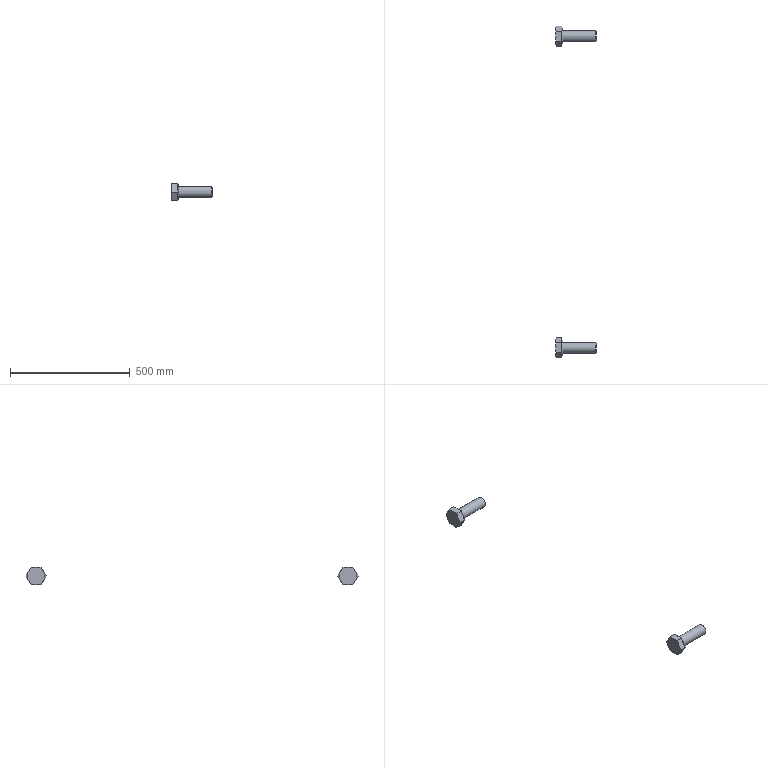Part | NX | features 10.SLDPRT 2, Delete Body 1, LINKED_BODY 1, SCALE 1 | 2 solids | 38 faces | box 170.438 x 1384 x 73.125 mm | volume 715384 mm3 | plane 20 | cone 16 | cylinder 2 | commonest cylinder face diameters 45 x2
STEP:
#1=CARTESIAN_POINT('',(351.807,1380.604,39.509));
#2=VERTEX_POINT('',#1);
#3=CARTESIAN_POINT('',(351.807,1380.604,7.25));
#4=DIRECTION('',(-1.,0.,0.));
#5=DIRECTION('',(0.,0.,1.));
#6=AXIS2_PLACEMENT_3D('',#3,#4,#5);
#7=CIRCLE('',#6,32.259);
#8=EDGE_CURVE('',#2,#2,#7,.T.);
#9=ORIENTED_EDGE('',*,*,#8,.F.);
#10=EDGE_LOOP('',(#9));
#11=FACE_BOUND('',#10,.T.);
#12=CARTESIAN_POINT('',(351.807,1380.604,29.75));
#13=VERTEX_POINT('',#12);
#14=CARTESIAN_POINT('',(351.807,1380.604,7.25));
#15=DIRECTION('',(-1.,0.,0.));
#16=DIRECTION('',(0.,0.,1.));
#17=AXIS2_PLACEMENT_3D('',#14,#15,#16);
#18=CIRCLE('',#17,22.5);
#19=EDGE_CURVE('',#13,#13,#18,.F.);
#20=ORIENTED_EDGE('',*,*,#19,.F.);
#21=EDGE_LOOP('',(#20));
#22=FACE_BOUND('',#21,.T.);
#23=CARTESIAN_POINT('',(351.807,1359.495,43.812));
#24=DIRECTION('',(-1.,0.,0.));
#25=DIRECTION('',(0.,0.,1.));
#26=AXIS2_PLACEMENT_3D('',#23,#24,#25);
#27=PLANE('',#26);
#28=ADVANCED_FACE('',(#11,#22),#27,.F.);
#29=CARTESIAN_POINT('',(324.054,1338.386,7.25));
#30=VERTEX_POINT('',#29);
#31=CARTESIAN_POINT('',(321.995,1348.94,25.531));
#32=VERTEX_POINT('',#31);
#33=CARTESIAN_POINT('',(324.054,1338.386,7.25));
#34=CARTESIAN_POINT('',(322.773,1341.904,13.344));
#35=CARTESIAN_POINT('',(321.995,1345.422,19.438));
#36=CARTESIAN_POINT('',(321.995,1348.94,25.531));
#37=B_SPLINE_CURVE_WITH_KNOTS('',3,(#33,#34,#35,#36),.UNSPECIFIED.,.F.,.F.,(4,4),(0.000001299,0.02111),.UNSPECIFIED.);
#38=EDGE_CURVE('',#30,#32,#37,.T.);
#39=ORIENTED_EDGE('',*,*,#38,.F.);
#40=CARTESIAN_POINT('',(348.432,1338.386,7.25));
#41=VERTEX_POINT('',#40);
#42=CARTESIAN_POINT('',(351.807,1338.386,7.25));
#43=DIRECTION('',(-1.,0.,0.));
#44=VECTOR('',#43,1000.);
#45=LINE('',#42,#44);
#46=EDGE_CURVE('',#41,#30,#45,.T.);
#47=ORIENTED_EDGE('',*,*,#46,.F.);
#48=CARTESIAN_POINT('',(348.432,1359.495,43.812));
#49=VERTEX_POINT('',#48);
#50=CARTESIAN_POINT('',(348.432,1359.495,43.812));
#51=DIRECTION('',(0.,-0.5,-0.866));
#52=VECTOR('',#51,1000.);
#53=LINE('',#50,#52);
#54=EDGE_CURVE('',#49,#41,#53,.T.);
#55=ORIENTED_EDGE('',*,*,#54,.F.);
#56=CARTESIAN_POINT('',(324.054,1359.495,43.812));
#57=VERTEX_POINT('',#56);
#58=CARTESIAN_POINT('',(351.807,1359.495,43.812));
#59=DIRECTION('',(-1.,0.,0.));
#60=VECTOR('',#59,1000.);
#61=LINE('',#58,#60);
#62=EDGE_CURVE('',#49,#57,#61,.T.);
#63=ORIENTED_EDGE('',*,*,#62,.T.);
#64=CARTESIAN_POINT('',(321.995,1348.94,25.531));
#65=CARTESIAN_POINT('',(321.995,1352.459,31.625));
#66=CARTESIAN_POINT('',(322.773,1355.977,37.719));
#67=CARTESIAN_POINT('',(324.054,1359.495,43.813));
#68=B_SPLINE_CURVE_WITH_KNOTS('',3,(#64,#65,#66,#67),.UNSPECIFIED.,.F.,.F.,(4,4),(0.02111,0.04222),.UNSPECIFIED.);
#69=EDGE_CURVE('',#32,#57,#68,.T.);
#70=ORIENTED_EDGE('',*,*,#69,.F.);
#71=EDGE_LOOP('',(#39,#47,#55,#63,#70));
#72=FACE_BOUND('',#71,.T.);
#73=CARTESIAN_POINT('',(351.807,1359.495,43.812));
#74=DIRECTION('',(0.,0.866,-0.5));
#75=DIRECTION('',(0.,0.5,0.866));
#76=AXIS2_PLACEMENT_3D('',#73,#74,#75);
#77=PLANE('',#76);
#78=ADVANCED_FACE('',(#72),#77,.F.);
#79=CARTESIAN_POINT('',(324.054,1359.495,-29.312));
#80=VERTEX_POINT('',#79);
#81=CARTESIAN_POINT('',(321.995,1348.94,-11.031));
#82=VERTEX_POINT('',#81);
#83=CARTESIAN_POINT('',(324.054,1359.495,-29.312));
#84=CARTESIAN_POINT('',(322.773,1355.977,-23.219));
#85=CARTESIAN_POINT('',(321.995,1352.459,-17.125));
#86=CARTESIAN_POINT('',(321.995,1348.94,-11.031));
#87=B_SPLINE_CURVE_WITH_KNOTS('',3,(#83,#84,#85,#86),.UNSPECIFIED.,.F.,.F.,(4,4),(0.000001299,0.02111),.UNSPECIFIED.);
#88=EDGE_CURVE('',#80,#82,#87,.T.);
#89=ORIENTED_EDGE('',*,*,#88,.F.);
#90=CARTESIAN_POINT('',(348.432,1359.495,-29.312));
#91=VERTEX_POINT('',#90);
#92=CARTESIAN_POINT('',(351.807,1359.495,-29.312));
#93=DIRECTION('',(-1.,0.,0.));
#94=VECTOR('',#93,1000.);
#95=LINE('',#92,#94);
#96=EDGE_CURVE('',#91,#80,#95,.T.);
#97=ORIENTED_EDGE('',*,*,#96,.F.);
#98=CARTESIAN_POINT('',(348.432,1338.386,7.25));
#99=DIRECTION('',(0.,0.5,-0.866));
#100=VECTOR('',#99,1000.);
#101=LINE('',#98,#100);
#102=EDGE_CURVE('',#41,#91,#101,.T.);
#103=ORIENTED_EDGE('',*,*,#102,.F.);
#104=ORIENTED_EDGE('',*,*,#46,.T.);
#105=CARTESIAN_POINT('',(321.995,1348.94,-11.031));
#106=CARTESIAN_POINT('',(321.995,1345.422,-4.937));
#107=CARTESIAN_POINT('',(322.773,1341.904,1.156));
#108=CARTESIAN_POINT('',(324.054,1338.386,7.25));
#109=B_SPLINE_CURVE_WITH_KNOTS('',3,(#105,#106,#107,#108),.UNSPECIFIED.,.F.,.F.,(4,4),(0.02111,0.04222),.UNSPECIFIED.);
#110=EDGE_CURVE('',#82,#30,#109,.T.);
#111=ORIENTED_EDGE('',*,*,#110,.F.);
#112=EDGE_LOOP('',(#89,#97,#103,#104,#111));
#113=FACE_BOUND('',#112,.T.);
#114=CARTESIAN_POINT('',(351.807,1338.386,7.25));
#115=DIRECTION('',(0.,0.866,0.5));
#116=DIRECTION('',(0.,-0.5,0.866));
#117=AXIS2_PLACEMENT_3D('',#114,#115,#116);
#118=PLANE('',#117);
#119=ADVANCED_FACE('',(#113),#118,.F.);
#120=CARTESIAN_POINT('',(324.054,1401.714,-29.312));
#121=VERTEX_POINT('',#120);
#122=CARTESIAN_POINT('',(321.995,1380.604,-29.312));
#123=VERTEX_POINT('',#122);
#124=CARTESIAN_POINT('',(321.995,1380.604,-29.312));
#125=CARTESIAN_POINT('',(321.995,1387.655,-29.312));
#126=CARTESIAN_POINT('',(322.777,1394.696,-29.312));
#127=CARTESIAN_POINT('',(324.054,1401.714,-29.312));
#128=B_SPLINE_CURVE_WITH_KNOTS('',3,(#124,#125,#126,#127),.UNSPECIFIED.,.F.,.F.,(4,4),(0.05719,0.07852),.UNSPECIFIED.);
#129=EDGE_CURVE('',#121,#123,#128,.F.);
#130=ORIENTED_EDGE('',*,*,#129,.F.);
#131=CARTESIAN_POINT('',(348.432,1401.714,-29.312));
#132=VERTEX_POINT('',#131);
#133=CARTESIAN_POINT('',(351.807,1401.714,-29.312));
#134=DIRECTION('',(-1.,0.,0.));
#135=VECTOR('',#134,1000.);
#136=LINE('',#133,#135);
#137=EDGE_CURVE('',#132,#121,#136,.T.);
#138=ORIENTED_EDGE('',*,*,#137,.F.);
#139=CARTESIAN_POINT('',(348.432,1359.495,-29.312));
#140=DIRECTION('',(0.,1.,0.));
#141=VECTOR('',#140,1000.);
#142=LINE('',#139,#141);
#143=EDGE_CURVE('',#91,#132,#142,.T.);
#144=ORIENTED_EDGE('',*,*,#143,.F.);
#145=ORIENTED_EDGE('',*,*,#96,.T.);
#146=CARTESIAN_POINT('',(324.054,1359.495,-29.312));
#147=CARTESIAN_POINT('',(322.782,1366.485,-29.312));
#148=CARTESIAN_POINT('',(321.995,1373.574,-29.312));
#149=CARTESIAN_POINT('',(321.995,1380.604,-29.312));
#150=B_SPLINE_CURVE_WITH_KNOTS('',3,(#146,#147,#148,#149),.UNSPECIFIED.,.F.,.F.,(4,4),(0.03591,0.05719),.UNSPECIFIED.);
#151=EDGE_CURVE('',#123,#80,#150,.F.);
#152=ORIENTED_EDGE('',*,*,#151,.F.);
#153=EDGE_LOOP('',(#130,#138,#144,#145,#152));
#154=FACE_BOUND('',#153,.T.);
#155=CARTESIAN_POINT('',(351.807,1359.495,-29.312));
#156=DIRECTION('',(0.,0.,1.));
#157=DIRECTION('',(0.,-1.,0.));
#158=AXIS2_PLACEMENT_3D('',#155,#156,#157);
#159=PLANE('',#158);
#160=ADVANCED_FACE('',(#154),#159,.F.);
#161=CARTESIAN_POINT('',(324.054,1422.823,7.25));
#162=VERTEX_POINT('',#161);
#163=CARTESIAN_POINT('',(321.995,1412.268,-11.031));
#164=VERTEX_POINT('',#163);
#165=CARTESIAN_POINT('',(324.054,1422.823,7.25));
#166=CARTESIAN_POINT('',(322.773,1419.305,1.156));
#167=CARTESIAN_POINT('',(321.995,1415.787,-4.938));
#168=CARTESIAN_POINT('',(321.995,1412.268,-11.031));
#169=B_SPLINE_CURVE_WITH_KNOTS('',3,(#165,#166,#167,#168),.UNSPECIFIED.,.F.,.F.,(4,4),(0.000001299,0.02111),.UNSPECIFIED.);
#170=EDGE_CURVE('',#162,#164,#169,.T.);
#171=ORIENTED_EDGE('',*,*,#170,.F.);
#172=CARTESIAN_POINT('',(348.432,1422.823,7.25));
#173=VERTEX_POINT('',#172);
#174=CARTESIAN_POINT('',(351.807,1422.823,7.25));
#175=DIRECTION('',(-1.,0.,0.));
#176=VECTOR('',#175,1000.);
#177=LINE('',#174,#176);
#178=EDGE_CURVE('',#173,#162,#177,.T.);
#179=ORIENTED_EDGE('',*,*,#178,.F.);
#180=CARTESIAN_POINT('',(348.432,1401.714,-29.312));
#181=DIRECTION('',(0.,0.5,0.866));
#182=VECTOR('',#181,1000.);
#183=LINE('',#180,#182);
#184=EDGE_CURVE('',#132,#173,#183,.T.);
#185=ORIENTED_EDGE('',*,*,#184,.F.);
#186=ORIENTED_EDGE('',*,*,#137,.T.);
#187=CARTESIAN_POINT('',(321.995,1412.268,-11.031));
#188=CARTESIAN_POINT('',(321.995,1408.75,-17.125));
#189=CARTESIAN_POINT('',(322.773,1405.232,-23.219));
#190=CARTESIAN_POINT('',(324.054,1401.714,-29.312));
#191=B_SPLINE_CURVE_WITH_KNOTS('',3,(#187,#188,#189,#190),.UNSPECIFIED.,.F.,.F.,(4,4),(0.02111,0.04222),.UNSPECIFIED.);
#192=EDGE_CURVE('',#164,#121,#191,.T.);
#193=ORIENTED_EDGE('',*,*,#192,.F.);
#194=EDGE_LOOP('',(#171,#179,#185,#186,#193));
#195=FACE_BOUND('',#194,.T.);
#196=CARTESIAN_POINT('',(351.807,1401.714,-29.312));
#197=DIRECTION('',(0.,-0.866,0.5));
#198=DIRECTION('',(0.,-0.5,-0.866));
#199=AXIS2_PLACEMENT_3D('',#196,#197,#198);
#200=PLANE('',#199);
#201=ADVANCED_FACE('',(#195),#200,.F.);
#202=CARTESIAN_POINT('',(324.054,1401.714,43.812));
#203=VERTEX_POINT('',#202);
#204=CARTESIAN_POINT('',(321.995,1412.268,25.531));
#205=VERTEX_POINT('',#204);
#206=CARTESIAN_POINT('',(324.054,1401.714,43.812));
#207=CARTESIAN_POINT('',(322.773,1405.232,37.719));
#208=CARTESIAN_POINT('',(321.995,1408.75,31.625));
#209=CARTESIAN_POINT('',(321.995,1412.268,25.531));
#210=B_SPLINE_CURVE_WITH_KNOTS('',3,(#206,#207,#208,#209),.UNSPECIFIED.,.F.,.F.,(4,4),(0.000001299,0.02111),.UNSPECIFIED.);
#211=EDGE_CURVE('',#203,#205,#210,.T.);
#212=ORIENTED_EDGE('',*,*,#211,.F.);
#213=CARTESIAN_POINT('',(348.432,1401.714,43.812));
#214=VERTEX_POINT('',#213);
#215=CARTESIAN_POINT('',(351.807,1401.714,43.812));
#216=DIRECTION('',(-1.,0.,0.));
#217=VECTOR('',#216,1000.);
#218=LINE('',#215,#217);
#219=EDGE_CURVE('',#214,#203,#218,.T.);
#220=ORIENTED_EDGE('',*,*,#219,.F.);
#221=CARTESIAN_POINT('',(348.432,1422.823,7.25));
#222=DIRECTION('',(0.,-0.5,0.866));
#223=VECTOR('',#222,1000.);
#224=LINE('',#221,#223);
#225=EDGE_CURVE('',#173,#214,#224,.T.);
#226=ORIENTED_EDGE('',*,*,#225,.F.);
#227=ORIENTED_EDGE('',*,*,#178,.T.);
#228=CARTESIAN_POINT('',(321.995,1412.268,25.531));
#229=CARTESIAN_POINT('',(321.995,1415.787,19.438));
#230=CARTESIAN_POINT('',(322.773,1419.305,13.344));
#231=CARTESIAN_POINT('',(324.054,1422.823,7.25));
#232=B_SPLINE_CURVE_WITH_KNOTS('',3,(#228,#229,#230,#231),.UNSPECIFIED.,.F.,.F.,(4,4),(0.02111,0.04222),.UNSPECIFIED.);
#233=EDGE_CURVE('',#205,#162,#232,.T.);
#234=ORIENTED_EDGE('',*,*,#233,.F.);
#235=EDGE_LOOP('',(#212,#220,#226,#227,#234));
#236=FACE_BOUND('',#235,.T.);
#237=CARTESIAN_POINT('',(351.807,1422.823,7.25));
#238=DIRECTION('',(0.,-0.866,-0.5));
#239=DIRECTION('',(0.,0.5,-0.866));
#240=AXIS2_PLACEMENT_3D('',#237,#238,#239);
#241=PLANE('',#240);
#242=ADVANCED_FACE('',(#236),#241,.F.);
#243=CARTESIAN_POINT('',(321.995,1380.604,43.812));
#244=VERTEX_POINT('',#243);
#245=CARTESIAN_POINT('',(324.054,1359.495,43.812));
#246=CARTESIAN_POINT('',(322.782,1366.485,43.812));
#247=CARTESIAN_POINT('',(321.995,1373.574,43.812));
#248=CARTESIAN_POINT('',(321.995,1380.604,43.812));
#249=B_SPLINE_CURVE_WITH_KNOTS('',3,(#245,#246,#247,#248),.UNSPECIFIED.,.F.,.F.,(4,4),(0.03591,0.05719),.UNSPECIFIED.);
#250=EDGE_CURVE('',#57,#244,#249,.T.);
#251=ORIENTED_EDGE('',*,*,#250,.F.);
#252=ORIENTED_EDGE('',*,*,#62,.F.);
#253=CARTESIAN_POINT('',(348.432,1401.714,43.812));
#254=DIRECTION('',(0.,-1.,0.));
#255=VECTOR('',#254,1000.);
#256=LINE('',#253,#255);
#257=EDGE_CURVE('',#214,#49,#256,.T.);
#258=ORIENTED_EDGE('',*,*,#257,.F.);
#259=ORIENTED_EDGE('',*,*,#219,.T.);
#260=CARTESIAN_POINT('',(321.995,1380.604,43.812));
#261=CARTESIAN_POINT('',(321.995,1387.655,43.812));
#262=CARTESIAN_POINT('',(322.777,1394.696,43.812));
#263=CARTESIAN_POINT('',(324.054,1401.714,43.812));
#264=B_SPLINE_CURVE_WITH_KNOTS('',3,(#260,#261,#262,#263),.UNSPECIFIED.,.F.,.F.,(4,4),(0.05719,0.07852),.UNSPECIFIED.);
#265=EDGE_CURVE('',#244,#203,#264,.T.);
#266=ORIENTED_EDGE('',*,*,#265,.F.);
#267=EDGE_LOOP('',(#251,#252,#258,#259,#266));
#268=FACE_BOUND('',#267,.T.);
#269=CARTESIAN_POINT('',(351.807,1401.714,43.812));
#270=DIRECTION('',(0.,0.,-1.));
#271=DIRECTION('',(-1.,0.,0.));
#272=AXIS2_PLACEMENT_3D('',#269,#270,#271);
#273=PLANE('',#272);
#274=ADVANCED_FACE('',(#268),#273,.F.);
#275=CARTESIAN_POINT('',(348.432,1380.604,42.884));
#276=VERTEX_POINT('',#275);
#277=CARTESIAN_POINT('',(348.432,1380.604,7.25));
#278=DIRECTION('',(-1.,0.,0.));
#279=DIRECTION('',(0.,0.,1.));
#280=AXIS2_PLACEMENT_3D('',#277,#278,#279);
#281=CIRCLE('',#280,35.634);
#282=EDGE_CURVE('',#276,#276,#281,.T.);
#283=ORIENTED_EDGE('',*,*,#282,.T.);
#284=EDGE_LOOP('',(#283));
#285=FACE_BOUND('',#284,.T.);
#286=ORIENTED_EDGE('',*,*,#54,.T.);
#287=ORIENTED_EDGE('',*,*,#102,.T.);
#288=ORIENTED_EDGE('',*,*,#143,.T.);
#289=ORIENTED_EDGE('',*,*,#184,.T.);
#290=ORIENTED_EDGE('',*,*,#225,.T.);
#291=ORIENTED_EDGE('',*,*,#257,.T.);
#292=EDGE_LOOP('',(#286,#287,#288,#289,#290,#291));
#293=FACE_BOUND('',#292,.T.);
#294=CARTESIAN_POINT('',(348.432,1416.239,7.25));
#295=DIRECTION('',(1.,0.,0.));
#296=DIRECTION('',(0.,0.,-1.));
#297=AXIS2_PLACEMENT_3D('',#294,#295,#296);
#298=PLANE('',#297);
#299=ADVANCED_FACE('',(#285,#293),#298,.T.);
#300=ORIENTED_EDGE('',*,*,#8,.T.);
#301=EDGE_LOOP('',(#300));
#302=FACE_BOUND('',#301,.T.);
#303=ORIENTED_EDGE('',*,*,#282,.F.);
#304=EDGE_LOOP('',(#303));
#305=FACE_BOUND('',#304,.T.);
#306=CARTESIAN_POINT('',(348.432,1380.604,7.25));
#307=DIRECTION('',(-1.,0.,0.));
#308=DIRECTION('',(0.,0.,1.));
#309=AXIS2_PLACEMENT_3D('',#306,#307,#308);
#310=CONICAL_SURFACE('',#309,35.634,0.7854);
#311=ADVANCED_FACE('',(#302,#305),#310,.T.);
#312=ORIENTED_EDGE('',*,*,#69,.T.);
#313=ORIENTED_EDGE('',*,*,#250,.T.);
#314=CARTESIAN_POINT('',(321.995,1380.604,7.25));
#315=DIRECTION('',(-1.,0.,0.));
#316=DIRECTION('',(0.,0.,1.));
#317=AXIS2_PLACEMENT_3D('',#314,#315,#316);
#318=CIRCLE('',#317,36.562);
#319=EDGE_CURVE('',#32,#244,#318,.T.);
#320=ORIENTED_EDGE('',*,*,#319,.F.);
#321=EDGE_LOOP('',(#312,#313,#320));
#322=FACE_BOUND('',#321,.T.);
#323=CARTESIAN_POINT('',(321.995,1380.604,7.25));
#324=DIRECTION('',(1.,0.,0.));
#325=DIRECTION('',(0.,0.,-1.));
#326=AXIS2_PLACEMENT_3D('',#323,#324,#325);
#327=CONICAL_SURFACE('',#326,36.562,1.222);
#328=ADVANCED_FACE('',(#322),#327,.T.);
#329=ORIENTED_EDGE('',*,*,#110,.T.);
#330=ORIENTED_EDGE('',*,*,#38,.T.);
#331=CARTESIAN_POINT('',(321.995,1380.604,7.25));
#332=DIRECTION('',(-1.,0.,0.));
#333=DIRECTION('',(0.,0.,1.));
#334=AXIS2_PLACEMENT_3D('',#331,#332,#333);
#335=CIRCLE('',#334,36.562);
#336=EDGE_CURVE('',#82,#32,#335,.T.);
#337=ORIENTED_EDGE('',*,*,#336,.F.);
#338=EDGE_LOOP('',(#329,#330,#337));
#339=FACE_BOUND('',#338,.T.);
#340=CARTESIAN_POINT('',(321.995,1380.604,7.25));
#341=DIRECTION('',(1.,0.,0.));
#342=DIRECTION('',(0.,0.,-1.));
#343=AXIS2_PLACEMENT_3D('',#340,#341,#342);
#344=CONICAL_SURFACE('',#343,36.562,1.222);
#345=ADVANCED_FACE('',(#339),#344,.T.);
#346=ORIENTED_EDGE('',*,*,#151,.T.);
#347=ORIENTED_EDGE('',*,*,#88,.T.);
#348=CARTESIAN_POINT('',(321.995,1380.604,7.25));
#349=DIRECTION('',(-1.,0.,0.));
#350=DIRECTION('',(0.,0.,1.));
#351=AXIS2_PLACEMENT_3D('',#348,#349,#350);
#352=CIRCLE('',#351,36.562);
#353=EDGE_CURVE('',#123,#82,#352,.T.);
#354=ORIENTED_EDGE('',*,*,#353,.F.);
#355=EDGE_LOOP('',(#346,#347,#354));
#356=FACE_BOUND('',#355,.T.);
#357=CARTESIAN_POINT('',(321.995,1380.604,7.25));
#358=DIRECTION('',(1.,0.,0.));
#359=DIRECTION('',(0.,0.,-1.));
#360=AXIS2_PLACEMENT_3D('',#357,#358,#359);
#361=CONICAL_SURFACE('',#360,36.562,1.222);
#362=ADVANCED_FACE('',(#356),#361,.T.);
#363=ORIENTED_EDGE('',*,*,#129,.T.);
#364=CARTESIAN_POINT('',(321.995,1380.604,7.25));
#365=DIRECTION('',(-1.,0.,0.));
#366=DIRECTION('',(0.,0.,1.));
#367=AXIS2_PLACEMENT_3D('',#364,#365,#366);
#368=CIRCLE('',#367,36.562);
#369=EDGE_CURVE('',#164,#123,#368,.T.);
#370=ORIENTED_EDGE('',*,*,#369,.F.);
#371=ORIENTED_EDGE('',*,*,#192,.T.);
#372=EDGE_LOOP('',(#363,#370,#371));
#373=FACE_BOUND('',#372,.T.);
#374=CARTESIAN_POINT('',(321.995,1380.604,7.25));
#375=DIRECTION('',(1.,0.,0.));
#376=DIRECTION('',(0.,0.,-1.));
#377=AXIS2_PLACEMENT_3D('',#374,#375,#376);
#378=CONICAL_SURFACE('',#377,36.562,1.222);
#379=ADVANCED_FACE('',(#373),#378,.T.);
#380=ORIENTED_EDGE('',*,*,#170,.T.);
#381=CARTESIAN_POINT('',(321.995,1380.604,7.25));
#382=DIRECTION('',(-1.,0.,0.));
#383=DIRECTION('',(0.,0.,1.));
#384=AXIS2_PLACEMENT_3D('',#381,#382,#383);
#385=CIRCLE('',#384,36.562);
#386=EDGE_CURVE('',#205,#164,#385,.T.);
#387=ORIENTED_EDGE('',*,*,#386,.F.);
#388=ORIENTED_EDGE('',*,*,#233,.T.);
#389=EDGE_LOOP('',(#380,#387,#388));
#390=FACE_BOUND('',#389,.T.);
#391=CARTESIAN_POINT('',(321.995,1380.604,7.25));
#392=DIRECTION('',(1.,0.,0.));
#393=DIRECTION('',(0.,0.,-1.));
#394=AXIS2_PLACEMENT_3D('',#391,#392,#393);
#395=CONICAL_SURFACE('',#394,36.562,1.222);
#396=ADVANCED_FACE('',(#390),#395,.T.);
#397=ORIENTED_EDGE('',*,*,#211,.T.);
#398=CARTESIAN_POINT('',(321.995,1380.604,7.25));
#399=DIRECTION('',(-1.,0.,0.));
#400=DIRECTION('',(0.,0.,1.));
#401=AXIS2_PLACEMENT_3D('',#398,#399,#400);
#402=CIRCLE('',#401,36.562);
#403=EDGE_CURVE('',#244,#205,#402,.T.);
#404=ORIENTED_EDGE('',*,*,#403,.F.);
#405=ORIENTED_EDGE('',*,*,#265,.T.);
#406=EDGE_LOOP('',(#397,#404,#405));
#407=FACE_BOUND('',#406,.T.);
#408=CARTESIAN_POINT('',(321.995,1380.604,7.25));
#409=DIRECTION('',(1.,0.,0.));
#410=DIRECTION('',(0.,0.,-1.));
#411=AXIS2_PLACEMENT_3D('',#408,#409,#410);
#412=CONICAL_SURFACE('',#411,36.562,1.222);
#413=ADVANCED_FACE('',(#407),#412,.T.);
#414=ORIENTED_EDGE('',*,*,#319,.T.);
#415=ORIENTED_EDGE('',*,*,#403,.T.);
#416=ORIENTED_EDGE('',*,*,#386,.T.);
#417=ORIENTED_EDGE('',*,*,#369,.T.);
#418=ORIENTED_EDGE('',*,*,#353,.T.);
#419=ORIENTED_EDGE('',*,*,#336,.T.);
#420=EDGE_LOOP('',(#414,#415,#416,#417,#418,#419));
#421=FACE_BOUND('',#420,.T.);
#422=CARTESIAN_POINT('',(321.995,1359.495,43.812));
#423=DIRECTION('',(-1.,0.,0.));
#424=DIRECTION('',(0.,0.,1.));
#425=AXIS2_PLACEMENT_3D('',#422,#423,#424);
#426=PLANE('',#425);
#427=ADVANCED_FACE('',(#421),#426,.T.);
#428=CARTESIAN_POINT('',(490.182,1380.604,-15.25));
#429=VERTEX_POINT('',#428);
#430=CARTESIAN_POINT('',(490.182,1380.604,7.25));
#431=DIRECTION('',(1.,0.,0.));
#432=DIRECTION('',(0.,0.,-1.));
#433=AXIS2_PLACEMENT_3D('',#430,#431,#432);
#434=CIRCLE('',#433,22.5);
#435=EDGE_CURVE('',#429,#429,#434,.F.);
#436=ORIENTED_EDGE('',*,*,#435,.T.);
#437=EDGE_LOOP('',(#436));
#438=FACE_BOUND('',#437,.T.);
#439=ORIENTED_EDGE('',*,*,#19,.T.);
#440=EDGE_LOOP('',(#439));
#441=FACE_BOUND('',#440,.T.);
#442=CARTESIAN_POINT('',(492.432,1380.604,7.25));
#443=DIRECTION('',(-1.,0.,0.));
#444=DIRECTION('',(0.,0.,1.));
#445=AXIS2_PLACEMENT_3D('',#442,#443,#444);
#446=CYLINDRICAL_SURFACE('',#445,22.5);
#447=ADVANCED_FACE('',(#438,#441),#446,.T.);
#448=CARTESIAN_POINT('',(492.432,1380.604,-13.));
#449=VERTEX_POINT('',#448);
#450=CARTESIAN_POINT('',(492.432,1380.604,7.25));
#451=DIRECTION('',(1.,0.,0.));
#452=DIRECTION('',(0.,0.,-1.));
#453=AXIS2_PLACEMENT_3D('',#450,#451,#452);
#454=CIRCLE('',#453,20.25);
#455=EDGE_CURVE('',#449,#449,#454,.T.);
#456=ORIENTED_EDGE('',*,*,#455,.T.);
#457=EDGE_LOOP('',(#456));
#458=FACE_BOUND('',#457,.T.);
#459=CARTESIAN_POINT('',(492.432,1380.604,7.25));
#460=DIRECTION('',(1.,0.,0.));
#461=DIRECTION('',(0.,0.,-1.));
#462=AXIS2_PLACEMENT_3D('',#459,#460,#461);
#463=PLANE('',#462);
#464=ADVANCED_FACE('',(#458),#463,.T.);
#465=ORIENTED_EDGE('',*,*,#435,.F.);
#466=EDGE_LOOP('',(#465));
#467=FACE_BOUND('',#466,.T.);
#468=ORIENTED_EDGE('',*,*,#455,.F.);
#469=EDGE_LOOP('',(#468));
#470=FACE_BOUND('',#469,.T.);
#471=CARTESIAN_POINT('',(492.432,1380.604,7.25));
#472=DIRECTION('',(-1.,0.,0.));
#473=DIRECTION('',(0.,0.,1.));
#474=AXIS2_PLACEMENT_3D('',#471,#472,#473);
#475=CONICAL_SURFACE('',#474,20.25,0.7854);
#476=ADVANCED_FACE('',(#467,#470),#475,.T.);
#477=CLOSED_SHELL('',(#28,#78,#119,#160,#201,#242,#274,#299,#311,#328,#345,#362,#379,#396,#413,#427,#447,#464,#476));
#478=MANIFOLD_SOLID_BREP('',#477);
#479=CARTESIAN_POINT('',(351.807,2679.979,39.509));
#480=VERTEX_POINT('',#479);
#481=CARTESIAN_POINT('',(351.807,2679.979,7.25));
#482=DIRECTION('',(-1.,0.,0.));
#483=DIRECTION('',(0.,0.,1.));
#484=AXIS2_PLACEMENT_3D('',#481,#482,#483);
#485=CIRCLE('',#484,32.259);
#486=EDGE_CURVE('',#480,#480,#485,.T.);
#487=ORIENTED_EDGE('',*,*,#486,.F.);
#488=EDGE_LOOP('',(#487));
#489=FACE_BOUND('',#488,.T.);
#490=CARTESIAN_POINT('',(351.807,2679.979,29.75));
#491=VERTEX_POINT('',#490);
#492=CARTESIAN_POINT('',(351.807,2679.979,7.25));
#493=DIRECTION('',(-1.,0.,0.));
#494=DIRECTION('',(0.,0.,1.));
#495=AXIS2_PLACEMENT_3D('',#492,#493,#494);
#496=CIRCLE('',#495,22.5);
#497=EDGE_CURVE('',#491,#491,#496,.F.);
#498=ORIENTED_EDGE('',*,*,#497,.F.);
#499=EDGE_LOOP('',(#498));
#500=FACE_BOUND('',#499,.T.);
#501=CARTESIAN_POINT('',(351.807,2658.87,43.813));
#502=DIRECTION('',(-1.,0.,0.));
#503=DIRECTION('',(0.,0.,1.));
#504=AXIS2_PLACEMENT_3D('',#501,#502,#503);
#505=PLANE('',#504);
#506=ADVANCED_FACE('',(#489,#500),#505,.F.);
#507=CARTESIAN_POINT('',(324.054,2637.761,7.25));
#508=VERTEX_POINT('',#507);
#509=CARTESIAN_POINT('',(321.995,2648.315,25.531));
#510=VERTEX_POINT('',#509);
#511=CARTESIAN_POINT('',(324.054,2637.761,7.25));
#512=CARTESIAN_POINT('',(322.773,2641.279,13.344));
#513=CARTESIAN_POINT('',(321.995,2644.797,19.437));
#514=CARTESIAN_POINT('',(321.995,2648.315,25.531));
#515=B_SPLINE_CURVE_WITH_KNOTS('',3,(#511,#512,#513,#514),.UNSPECIFIED.,.F.,.F.,(4,4),(0.000001299,0.02111),.UNSPECIFIED.);
#516=EDGE_CURVE('',#508,#510,#515,.T.);
#517=ORIENTED_EDGE('',*,*,#516,.F.);
#518=CARTESIAN_POINT('',(348.432,2637.761,7.25));
#519=VERTEX_POINT('',#518);
#520=CARTESIAN_POINT('',(351.807,2637.761,7.25));
#521=DIRECTION('',(-1.,0.,0.));
#522=VECTOR('',#521,1000.);
#523=LINE('',#520,#522);
#524=EDGE_CURVE('',#519,#508,#523,.T.);
#525=ORIENTED_EDGE('',*,*,#524,.F.);
#526=CARTESIAN_POINT('',(348.432,2658.87,43.813));
#527=VERTEX_POINT('',#526);
#528=CARTESIAN_POINT('',(348.432,2658.87,43.813));
#529=DIRECTION('',(0.,-0.5,-0.866));
#530=VECTOR('',#529,1000.);
#531=LINE('',#528,#530);
#532=EDGE_CURVE('',#527,#519,#531,.T.);
#533=ORIENTED_EDGE('',*,*,#532,.F.);
#534=CARTESIAN_POINT('',(324.054,2658.87,43.813));
#535=VERTEX_POINT('',#534);
#536=CARTESIAN_POINT('',(351.807,2658.87,43.813));
#537=DIRECTION('',(-1.,0.,0.));
#538=VECTOR('',#537,1000.);
#539=LINE('',#536,#538);
#540=EDGE_CURVE('',#527,#535,#539,.T.);
#541=ORIENTED_EDGE('',*,*,#540,.T.);
#542=CARTESIAN_POINT('',(321.995,2648.315,25.531));
#543=CARTESIAN_POINT('',(321.995,2651.834,31.625));
#544=CARTESIAN_POINT('',(322.773,2655.352,37.719));
#545=CARTESIAN_POINT('',(324.054,2658.87,43.813));
#546=B_SPLINE_CURVE_WITH_KNOTS('',3,(#542,#543,#544,#545),.UNSPECIFIED.,.F.,.F.,(4,4),(0.02111,0.04222),.UNSPECIFIED.);
#547=EDGE_CURVE('',#510,#535,#546,.T.);
#548=ORIENTED_EDGE('',*,*,#547,.F.);
#549=EDGE_LOOP('',(#517,#525,#533,#541,#548));
#550=FACE_BOUND('',#549,.T.);
#551=CARTESIAN_POINT('',(351.807,2658.87,43.813));
#552=DIRECTION('',(0.,0.866,-0.5));
#553=DIRECTION('',(0.,0.5,0.866));
#554=AXIS2_PLACEMENT_3D('',#551,#552,#553);
#555=PLANE('',#554);
#556=ADVANCED_FACE('',(#550),#555,.F.);
#557=CARTESIAN_POINT('',(324.054,2658.87,-29.312));
#558=VERTEX_POINT('',#557);
#559=CARTESIAN_POINT('',(321.995,2648.315,-11.031));
#560=VERTEX_POINT('',#559);
#561=CARTESIAN_POINT('',(324.054,2658.87,-29.312));
#562=CARTESIAN_POINT('',(322.773,2655.352,-23.219));
#563=CARTESIAN_POINT('',(321.995,2651.834,-17.125));
#564=CARTESIAN_POINT('',(321.995,2648.315,-11.031));
#565=B_SPLINE_CURVE_WITH_KNOTS('',3,(#561,#562,#563,#564),.UNSPECIFIED.,.F.,.F.,(4,4),(0.000001299,0.02111),.UNSPECIFIED.);
#566=EDGE_CURVE('',#558,#560,#565,.T.);
#567=ORIENTED_EDGE('',*,*,#566,.F.);
#568=CARTESIAN_POINT('',(348.432,2658.87,-29.312));
#569=VERTEX_POINT('',#568);
#570=CARTESIAN_POINT('',(351.807,2658.87,-29.312));
#571=DIRECTION('',(-1.,0.,0.));
#572=VECTOR('',#571,1000.);
#573=LINE('',#570,#572);
#574=EDGE_CURVE('',#569,#558,#573,.T.);
#575=ORIENTED_EDGE('',*,*,#574,.F.);
#576=CARTESIAN_POINT('',(348.432,2637.761,7.25));
#577=DIRECTION('',(0.,0.5,-0.866));
#578=VECTOR('',#577,1000.);
#579=LINE('',#576,#578);
#580=EDGE_CURVE('',#519,#569,#579,.T.);
#581=ORIENTED_EDGE('',*,*,#580,.F.);
#582=ORIENTED_EDGE('',*,*,#524,.T.);
#583=CARTESIAN_POINT('',(321.995,2648.315,-11.031));
#584=CARTESIAN_POINT('',(321.995,2644.797,-4.937));
#585=CARTESIAN_POINT('',(322.773,2641.279,1.156));
#586=CARTESIAN_POINT('',(324.054,2637.761,7.25));
#587=B_SPLINE_CURVE_WITH_KNOTS('',3,(#583,#584,#585,#586),.UNSPECIFIED.,.F.,.F.,(4,4),(0.02111,0.04222),.UNSPECIFIED.);
#588=EDGE_CURVE('',#560,#508,#587,.T.);
#589=ORIENTED_EDGE('',*,*,#588,.F.);
#590=EDGE_LOOP('',(#567,#575,#581,#582,#589));
#591=FACE_BOUND('',#590,.T.);
#592=CARTESIAN_POINT('',(351.807,2637.761,7.25));
#593=DIRECTION('',(0.,0.866,0.5));
#594=DIRECTION('',(0.,-0.5,0.866));
#595=AXIS2_PLACEMENT_3D('',#592,#593,#594);
#596=PLANE('',#595);
#597=ADVANCED_FACE('',(#591),#596,.F.);
#598=CARTESIAN_POINT('',(324.054,2701.089,-29.312));
#599=VERTEX_POINT('',#598);
#600=CARTESIAN_POINT('',(321.995,2679.979,-29.312));
#601=VERTEX_POINT('',#600);
#602=CARTESIAN_POINT('',(321.995,2679.979,-29.312));
#603=CARTESIAN_POINT('',(321.995,2687.03,-29.312));
#604=CARTESIAN_POINT('',(322.777,2694.071,-29.312));
#605=CARTESIAN_POINT('',(324.054,2701.089,-29.312));
#606=B_SPLINE_CURVE_WITH_KNOTS('',3,(#602,#603,#604,#605),.UNSPECIFIED.,.F.,.F.,(4,4),(0.05719,0.07852),.UNSPECIFIED.);
#607=EDGE_CURVE('',#599,#601,#606,.F.);
#608=ORIENTED_EDGE('',*,*,#607,.F.);
#609=CARTESIAN_POINT('',(348.432,2701.089,-29.312));
#610=VERTEX_POINT('',#609);
#611=CARTESIAN_POINT('',(351.807,2701.089,-29.312));
#612=DIRECTION('',(-1.,0.,0.));
#613=VECTOR('',#612,1000.);
#614=LINE('',#611,#613);
#615=EDGE_CURVE('',#610,#599,#614,.T.);
#616=ORIENTED_EDGE('',*,*,#615,.F.);
#617=CARTESIAN_POINT('',(348.432,2658.87,-29.312));
#618=DIRECTION('',(0.,1.,0.));
#619=VECTOR('',#618,1000.);
#620=LINE('',#617,#619);
#621=EDGE_CURVE('',#569,#610,#620,.T.);
#622=ORIENTED_EDGE('',*,*,#621,.F.);
#623=ORIENTED_EDGE('',*,*,#574,.T.);
#624=CARTESIAN_POINT('',(324.054,2658.87,-29.312));
#625=CARTESIAN_POINT('',(322.782,2665.86,-29.312));
#626=CARTESIAN_POINT('',(321.995,2672.949,-29.312));
#627=CARTESIAN_POINT('',(321.995,2679.979,-29.312));
#628=B_SPLINE_CURVE_WITH_KNOTS('',3,(#624,#625,#626,#627),.UNSPECIFIED.,.F.,.F.,(4,4),(0.03591,0.05719),.UNSPECIFIED.);
#629=EDGE_CURVE('',#601,#558,#628,.F.);
#630=ORIENTED_EDGE('',*,*,#629,.F.);
#631=EDGE_LOOP('',(#608,#616,#622,#623,#630));
#632=FACE_BOUND('',#631,.T.);
#633=CARTESIAN_POINT('',(351.807,2658.87,-29.312));
#634=DIRECTION('',(0.,0.,1.));
#635=DIRECTION('',(0.,-1.,0.));
#636=AXIS2_PLACEMENT_3D('',#633,#634,#635);
#637=PLANE('',#636);
#638=ADVANCED_FACE('',(#632),#637,.F.);
#639=CARTESIAN_POINT('',(324.054,2722.198,7.25));
#640=VERTEX_POINT('',#639);
#641=CARTESIAN_POINT('',(321.995,2711.643,-11.031));
#642=VERTEX_POINT('',#641);
#643=CARTESIAN_POINT('',(324.054,2722.198,7.25));
#644=CARTESIAN_POINT('',(322.773,2718.68,1.156));
#645=CARTESIAN_POINT('',(321.995,2715.162,-4.937));
#646=CARTESIAN_POINT('',(321.995,2711.643,-11.031));
#647=B_SPLINE_CURVE_WITH_KNOTS('',3,(#643,#644,#645,#646),.UNSPECIFIED.,.F.,.F.,(4,4),(0.000001299,0.02111),.UNSPECIFIED.);
#648=EDGE_CURVE('',#640,#642,#647,.T.);
#649=ORIENTED_EDGE('',*,*,#648,.F.);
#650=CARTESIAN_POINT('',(348.432,2722.198,7.25));
#651=VERTEX_POINT('',#650);
#652=CARTESIAN_POINT('',(351.807,2722.198,7.25));
#653=DIRECTION('',(-1.,0.,0.));
#654=VECTOR('',#653,1000.);
#655=LINE('',#652,#654);
#656=EDGE_CURVE('',#651,#640,#655,.T.);
#657=ORIENTED_EDGE('',*,*,#656,.F.);
#658=CARTESIAN_POINT('',(348.432,2701.089,-29.312));
#659=DIRECTION('',(0.,0.5,0.866));
#660=VECTOR('',#659,1000.);
#661=LINE('',#658,#660);
#662=EDGE_CURVE('',#610,#651,#661,.T.);
#663=ORIENTED_EDGE('',*,*,#662,.F.);
#664=ORIENTED_EDGE('',*,*,#615,.T.);
#665=CARTESIAN_POINT('',(321.995,2711.643,-11.031));
#666=CARTESIAN_POINT('',(321.995,2708.125,-17.125));
#667=CARTESIAN_POINT('',(322.773,2704.607,-23.219));
#668=CARTESIAN_POINT('',(324.054,2701.089,-29.312));
#669=B_SPLINE_CURVE_WITH_KNOTS('',3,(#665,#666,#667,#668),.UNSPECIFIED.,.F.,.F.,(4,4),(0.02111,0.04222),.UNSPECIFIED.);
#670=EDGE_CURVE('',#642,#599,#669,.T.);
#671=ORIENTED_EDGE('',*,*,#670,.F.);
#672=EDGE_LOOP('',(#649,#657,#663,#664,#671));
#673=FACE_BOUND('',#672,.T.);
#674=CARTESIAN_POINT('',(351.807,2701.089,-29.312));
#675=DIRECTION('',(0.,-0.866,0.5));
#676=DIRECTION('',(0.,-0.5,-0.866));
#677=AXIS2_PLACEMENT_3D('',#674,#675,#676);
#678=PLANE('',#677);
#679=ADVANCED_FACE('',(#673),#678,.F.);
#680=CARTESIAN_POINT('',(324.054,2701.089,43.813));
#681=VERTEX_POINT('',#680);
#682=CARTESIAN_POINT('',(321.995,2711.643,25.531));
#683=VERTEX_POINT('',#682);
#684=CARTESIAN_POINT('',(324.054,2701.089,43.813));
#685=CARTESIAN_POINT('',(322.773,2704.607,37.719));
#686=CARTESIAN_POINT('',(321.995,2708.125,31.625));
#687=CARTESIAN_POINT('',(321.995,2711.643,25.531));
#688=B_SPLINE_CURVE_WITH_KNOTS('',3,(#684,#685,#686,#687),.UNSPECIFIED.,.F.,.F.,(4,4),(0.000001299,0.02111),.UNSPECIFIED.);
#689=EDGE_CURVE('',#681,#683,#688,.T.);
#690=ORIENTED_EDGE('',*,*,#689,.F.);
#691=CARTESIAN_POINT('',(348.432,2701.089,43.813));
#692=VERTEX_POINT('',#691);
#693=CARTESIAN_POINT('',(351.807,2701.089,43.813));
#694=DIRECTION('',(-1.,0.,0.));
#695=VECTOR('',#694,1000.);
#696=LINE('',#693,#695);
#697=EDGE_CURVE('',#692,#681,#696,.T.);
#698=ORIENTED_EDGE('',*,*,#697,.F.);
#699=CARTESIAN_POINT('',(348.432,2722.198,7.25));
#700=DIRECTION('',(0.,-0.5,0.866));
#701=VECTOR('',#700,1000.);
#702=LINE('',#699,#701);
#703=EDGE_CURVE('',#651,#692,#702,.T.);
#704=ORIENTED_EDGE('',*,*,#703,.F.);
#705=ORIENTED_EDGE('',*,*,#656,.T.);
#706=CARTESIAN_POINT('',(321.995,2711.643,25.531));
#707=CARTESIAN_POINT('',(321.995,2715.162,19.438));
#708=CARTESIAN_POINT('',(322.773,2718.68,13.344));
#709=CARTESIAN_POINT('',(324.054,2722.198,7.25));
#710=B_SPLINE_CURVE_WITH_KNOTS('',3,(#706,#707,#708,#709),.UNSPECIFIED.,.F.,.F.,(4,4),(0.02111,0.04222),.UNSPECIFIED.);
#711=EDGE_CURVE('',#683,#640,#710,.T.);
#712=ORIENTED_EDGE('',*,*,#711,.F.);
#713=EDGE_LOOP('',(#690,#698,#704,#705,#712));
#714=FACE_BOUND('',#713,.T.);
#715=CARTESIAN_POINT('',(351.807,2722.198,7.25));
#716=DIRECTION('',(0.,-0.866,-0.5));
#717=DIRECTION('',(0.,0.5,-0.866));
#718=AXIS2_PLACEMENT_3D('',#715,#716,#717);
#719=PLANE('',#718);
#720=ADVANCED_FACE('',(#714),#719,.F.);
#721=CARTESIAN_POINT('',(321.995,2679.979,43.813));
#722=VERTEX_POINT('',#721);
#723=CARTESIAN_POINT('',(324.054,2658.87,43.813));
#724=CARTESIAN_POINT('',(322.782,2665.86,43.813));
#725=CARTESIAN_POINT('',(321.995,2672.949,43.813));
#726=CARTESIAN_POINT('',(321.995,2679.979,43.813));
#727=B_SPLINE_CURVE_WITH_KNOTS('',3,(#723,#724,#725,#726),.UNSPECIFIED.,.F.,.F.,(4,4),(0.03591,0.05719),.UNSPECIFIED.);
#728=EDGE_CURVE('',#535,#722,#727,.T.);
#729=ORIENTED_EDGE('',*,*,#728,.F.);
#730=ORIENTED_EDGE('',*,*,#540,.F.);
#731=CARTESIAN_POINT('',(348.432,2701.089,43.813));
#732=DIRECTION('',(0.,-1.,0.));
#733=VECTOR('',#732,1000.);
#734=LINE('',#731,#733);
#735=EDGE_CURVE('',#692,#527,#734,.T.);
#736=ORIENTED_EDGE('',*,*,#735,.F.);
#737=ORIENTED_EDGE('',*,*,#697,.T.);
#738=CARTESIAN_POINT('',(321.995,2679.979,43.813));
#739=CARTESIAN_POINT('',(321.995,2687.03,43.813));
#740=CARTESIAN_POINT('',(322.777,2694.071,43.813));
#741=CARTESIAN_POINT('',(324.054,2701.089,43.813));
#742=B_SPLINE_CURVE_WITH_KNOTS('',3,(#738,#739,#740,#741),.UNSPECIFIED.,.F.,.F.,(4,4),(0.05719,0.07852),.UNSPECIFIED.);
#743=EDGE_CURVE('',#722,#681,#742,.T.);
#744=ORIENTED_EDGE('',*,*,#743,.F.);
#745=EDGE_LOOP('',(#729,#730,#736,#737,#744));
#746=FACE_BOUND('',#745,.T.);
#747=CARTESIAN_POINT('',(351.807,2701.089,43.813));
#748=DIRECTION('',(0.,0.,-1.));
#749=DIRECTION('',(-1.,0.,0.));
#750=AXIS2_PLACEMENT_3D('',#747,#748,#749);
#751=PLANE('',#750);
#752=ADVANCED_FACE('',(#746),#751,.F.);
#753=CARTESIAN_POINT('',(348.432,2679.979,42.884));
#754=VERTEX_POINT('',#753);
#755=CARTESIAN_POINT('',(348.432,2679.979,7.25));
#756=DIRECTION('',(-1.,0.,0.));
#757=DIRECTION('',(0.,0.,1.));
#758=AXIS2_PLACEMENT_3D('',#755,#756,#757);
#759=CIRCLE('',#758,35.634);
#760=EDGE_CURVE('',#754,#754,#759,.T.);
#761=ORIENTED_EDGE('',*,*,#760,.T.);
#762=EDGE_LOOP('',(#761));
#763=FACE_BOUND('',#762,.T.);
#764=ORIENTED_EDGE('',*,*,#532,.T.);
#765=ORIENTED_EDGE('',*,*,#580,.T.);
#766=ORIENTED_EDGE('',*,*,#621,.T.);
#767=ORIENTED_EDGE('',*,*,#662,.T.);
#768=ORIENTED_EDGE('',*,*,#703,.T.);
#769=ORIENTED_EDGE('',*,*,#735,.T.);
#770=EDGE_LOOP('',(#764,#765,#766,#767,#768,#769));
#771=FACE_BOUND('',#770,.T.);
#772=CARTESIAN_POINT('',(348.432,2715.614,7.25));
#773=DIRECTION('',(1.,0.,0.));
#774=DIRECTION('',(0.,0.,-1.));
#775=AXIS2_PLACEMENT_3D('',#772,#773,#774);
#776=PLANE('',#775);
#777=ADVANCED_FACE('',(#763,#771),#776,.T.);
#778=ORIENTED_EDGE('',*,*,#486,.T.);
#779=EDGE_LOOP('',(#778));
#780=FACE_BOUND('',#779,.T.);
#781=ORIENTED_EDGE('',*,*,#760,.F.);
#782=EDGE_LOOP('',(#781));
#783=FACE_BOUND('',#782,.T.);
#784=CARTESIAN_POINT('',(348.432,2679.979,7.25));
#785=DIRECTION('',(-1.,0.,0.));
#786=DIRECTION('',(0.,0.,1.));
#787=AXIS2_PLACEMENT_3D('',#784,#785,#786);
#788=CONICAL_SURFACE('',#787,35.634,0.7854);
#789=ADVANCED_FACE('',(#780,#783),#788,.T.);
#790=ORIENTED_EDGE('',*,*,#547,.T.);
#791=ORIENTED_EDGE('',*,*,#728,.T.);
#792=CARTESIAN_POINT('',(321.995,2679.979,7.25));
#793=DIRECTION('',(-1.,0.,0.));
#794=DIRECTION('',(0.,0.,1.));
#795=AXIS2_PLACEMENT_3D('',#792,#793,#794);
#796=CIRCLE('',#795,36.562);
#797=EDGE_CURVE('',#510,#722,#796,.T.);
#798=ORIENTED_EDGE('',*,*,#797,.F.);
#799=EDGE_LOOP('',(#790,#791,#798));
#800=FACE_BOUND('',#799,.T.);
#801=CARTESIAN_POINT('',(321.995,2679.979,7.25));
#802=DIRECTION('',(1.,0.,0.));
#803=DIRECTION('',(0.,0.,-1.));
#804=AXIS2_PLACEMENT_3D('',#801,#802,#803);
#805=CONICAL_SURFACE('',#804,36.562,1.222);
#806=ADVANCED_FACE('',(#800),#805,.T.);
#807=ORIENTED_EDGE('',*,*,#588,.T.);
#808=ORIENTED_EDGE('',*,*,#516,.T.);
#809=CARTESIAN_POINT('',(321.995,2679.979,7.25));
#810=DIRECTION('',(-1.,0.,0.));
#811=DIRECTION('',(0.,0.,1.));
#812=AXIS2_PLACEMENT_3D('',#809,#810,#811);
#813=CIRCLE('',#812,36.562);
#814=EDGE_CURVE('',#560,#510,#813,.T.);
#815=ORIENTED_EDGE('',*,*,#814,.F.);
#816=EDGE_LOOP('',(#807,#808,#815));
#817=FACE_BOUND('',#816,.T.);
#818=CARTESIAN_POINT('',(321.995,2679.979,7.25));
#819=DIRECTION('',(1.,0.,0.));
#820=DIRECTION('',(0.,0.,-1.));
#821=AXIS2_PLACEMENT_3D('',#818,#819,#820);
#822=CONICAL_SURFACE('',#821,36.562,1.222);
#823=ADVANCED_FACE('',(#817),#822,.T.);
#824=ORIENTED_EDGE('',*,*,#629,.T.);
#825=ORIENTED_EDGE('',*,*,#566,.T.);
#826=CARTESIAN_POINT('',(321.995,2679.979,7.25));
#827=DIRECTION('',(-1.,0.,0.));
#828=DIRECTION('',(0.,0.,1.));
#829=AXIS2_PLACEMENT_3D('',#826,#827,#828);
#830=CIRCLE('',#829,36.562);
#831=EDGE_CURVE('',#601,#560,#830,.T.);
#832=ORIENTED_EDGE('',*,*,#831,.F.);
#833=EDGE_LOOP('',(#824,#825,#832));
#834=FACE_BOUND('',#833,.T.);
#835=CARTESIAN_POINT('',(321.995,2679.979,7.25));
#836=DIRECTION('',(1.,0.,0.));
#837=DIRECTION('',(0.,0.,-1.));
#838=AXIS2_PLACEMENT_3D('',#835,#836,#837);
#839=CONICAL_SURFACE('',#838,36.562,1.222);
#840=ADVANCED_FACE('',(#834),#839,.T.);
#841=ORIENTED_EDGE('',*,*,#607,.T.);
#842=CARTESIAN_POINT('',(321.995,2679.979,7.25));
#843=DIRECTION('',(-1.,0.,0.));
#844=DIRECTION('',(0.,0.,1.));
#845=AXIS2_PLACEMENT_3D('',#842,#843,#844);
#846=CIRCLE('',#845,36.562);
#847=EDGE_CURVE('',#642,#601,#846,.T.);
#848=ORIENTED_EDGE('',*,*,#847,.F.);
#849=ORIENTED_EDGE('',*,*,#670,.T.);
#850=EDGE_LOOP('',(#841,#848,#849));
#851=FACE_BOUND('',#850,.T.);
#852=CARTESIAN_POINT('',(321.995,2679.979,7.25));
#853=DIRECTION('',(1.,0.,0.));
#854=DIRECTION('',(0.,0.,-1.));
#855=AXIS2_PLACEMENT_3D('',#852,#853,#854);
#856=CONICAL_SURFACE('',#855,36.562,1.222);
#857=ADVANCED_FACE('',(#851),#856,.T.);
#858=ORIENTED_EDGE('',*,*,#648,.T.);
#859=CARTESIAN_POINT('',(321.995,2679.979,7.25));
#860=DIRECTION('',(-1.,0.,0.));
#861=DIRECTION('',(0.,0.,1.));
#862=AXIS2_PLACEMENT_3D('',#859,#860,#861);
#863=CIRCLE('',#862,36.562);
#864=EDGE_CURVE('',#683,#642,#863,.T.);
#865=ORIENTED_EDGE('',*,*,#864,.F.);
#866=ORIENTED_EDGE('',*,*,#711,.T.);
#867=EDGE_LOOP('',(#858,#865,#866));
#868=FACE_BOUND('',#867,.T.);
#869=CARTESIAN_POINT('',(321.995,2679.979,7.25));
#870=DIRECTION('',(1.,0.,0.));
#871=DIRECTION('',(0.,0.,-1.));
#872=AXIS2_PLACEMENT_3D('',#869,#870,#871);
#873=CONICAL_SURFACE('',#872,36.562,1.222);
#874=ADVANCED_FACE('',(#868),#873,.T.);
#875=ORIENTED_EDGE('',*,*,#689,.T.);
#876=CARTESIAN_POINT('',(321.995,2679.979,7.25));
#877=DIRECTION('',(-1.,0.,0.));
#878=DIRECTION('',(0.,0.,1.));
#879=AXIS2_PLACEMENT_3D('',#876,#877,#878);
#880=CIRCLE('',#879,36.562);
#881=EDGE_CURVE('',#722,#683,#880,.T.);
#882=ORIENTED_EDGE('',*,*,#881,.F.);
#883=ORIENTED_EDGE('',*,*,#743,.T.);
#884=EDGE_LOOP('',(#875,#882,#883));
#885=FACE_BOUND('',#884,.T.);
#886=CARTESIAN_POINT('',(321.995,2679.979,7.25));
#887=DIRECTION('',(1.,0.,0.));
#888=DIRECTION('',(0.,0.,-1.));
#889=AXIS2_PLACEMENT_3D('',#886,#887,#888);
#890=CONICAL_SURFACE('',#889,36.562,1.222);
#891=ADVANCED_FACE('',(#885),#890,.T.);
#892=ORIENTED_EDGE('',*,*,#797,.T.);
#893=ORIENTED_EDGE('',*,*,#881,.T.);
#894=ORIENTED_EDGE('',*,*,#864,.T.);
#895=ORIENTED_EDGE('',*,*,#847,.T.);
#896=ORIENTED_EDGE('',*,*,#831,.T.);
#897=ORIENTED_EDGE('',*,*,#814,.T.);
#898=EDGE_LOOP('',(#892,#893,#894,#895,#896,#897));
#899=FACE_BOUND('',#898,.T.);
#900=CARTESIAN_POINT('',(321.995,2658.87,43.813));
#901=DIRECTION('',(-1.,0.,0.));
#902=DIRECTION('',(0.,0.,1.));
#903=AXIS2_PLACEMENT_3D('',#900,#901,#902);
#904=PLANE('',#903);
#905=ADVANCED_FACE('',(#899),#904,.T.);
#906=CARTESIAN_POINT('',(490.182,2679.979,-15.25));
#907=VERTEX_POINT('',#906);
#908=CARTESIAN_POINT('',(490.182,2679.979,7.25));
#909=DIRECTION('',(1.,0.,0.));
#910=DIRECTION('',(0.,0.,-1.));
#911=AXIS2_PLACEMENT_3D('',#908,#909,#910);
#912=CIRCLE('',#911,22.5);
#913=EDGE_CURVE('',#907,#907,#912,.F.);
#914=ORIENTED_EDGE('',*,*,#913,.T.);
#915=EDGE_LOOP('',(#914));
#916=FACE_BOUND('',#915,.T.);
#917=ORIENTED_EDGE('',*,*,#497,.T.);
#918=EDGE_LOOP('',(#917));
#919=FACE_BOUND('',#918,.T.);
#920=CARTESIAN_POINT('',(492.432,2679.979,7.25));
#921=DIRECTION('',(-1.,0.,0.));
#922=DIRECTION('',(0.,0.,1.));
#923=AXIS2_PLACEMENT_3D('',#920,#921,#922);
#924=CYLINDRICAL_SURFACE('',#923,22.5);
#925=ADVANCED_FACE('',(#916,#919),#924,.T.);
#926=CARTESIAN_POINT('',(492.432,2679.979,-13.));
#927=VERTEX_POINT('',#926);
#928=CARTESIAN_POINT('',(492.432,2679.979,7.25));
#929=DIRECTION('',(1.,0.,0.));
#930=DIRECTION('',(0.,0.,-1.));
#931=AXIS2_PLACEMENT_3D('',#928,#929,#930);
#932=CIRCLE('',#931,20.25);
#933=EDGE_CURVE('',#927,#927,#932,.T.);
#934=ORIENTED_EDGE('',*,*,#933,.T.);
#935=EDGE_LOOP('',(#934));
#936=FACE_BOUND('',#935,.T.);
#937=CARTESIAN_POINT('',(492.432,2679.979,7.25));
#938=DIRECTION('',(1.,0.,0.));
#939=DIRECTION('',(0.,0.,-1.));
#940=AXIS2_PLACEMENT_3D('',#937,#938,#939);
#941=PLANE('',#940);
#942=ADVANCED_FACE('',(#936),#941,.T.);
#943=ORIENTED_EDGE('',*,*,#913,.F.);
#944=EDGE_LOOP('',(#943));
#945=FACE_BOUND('',#944,.T.);
#946=ORIENTED_EDGE('',*,*,#933,.F.);
#947=EDGE_LOOP('',(#946));
#948=FACE_BOUND('',#947,.T.);
#949=CARTESIAN_POINT('',(492.432,2679.979,7.25));
#950=DIRECTION('',(-1.,0.,0.));
#951=DIRECTION('',(0.,0.,1.));
#952=AXIS2_PLACEMENT_3D('',#949,#950,#951);
#953=CONICAL_SURFACE('',#952,20.25,0.7854);
#954=ADVANCED_FACE('',(#945,#948),#953,.T.);
#955=CLOSED_SHELL('',(#506,#556,#597,#638,#679,#720,#752,#777,#789,#806,#823,#840,#857,#874,#891,#905,#925,#942,#954));
#956=MANIFOLD_SOLID_BREP('',#955);
#957=(LENGTH_UNIT()NAMED_UNIT(*)SI_UNIT(.MILLI.,.METRE.));
#958=UNCERTAINTY_MEASURE_WITH_UNIT(LENGTH_MEASURE(0.0508),#957,'','');
#959=(NAMED_UNIT(*)PLANE_ANGLE_UNIT()SI_UNIT($,.RADIAN.));
#960=(NAMED_UNIT(*)SI_UNIT($,.STERADIAN.)SOLID_ANGLE_UNIT());
#961=(GEOMETRIC_REPRESENTATION_CONTEXT(3)GLOBAL_UNCERTAINTY_ASSIGNED_CONTEXT((#958))GLOBAL_UNIT_ASSIGNED_CONTEXT((#957,#959,#960))REPRESENTATION_CONTEXT('',''));
#962=ADVANCED_BREP_SHAPE_REPRESENTATION('',(#478,#956),#961);